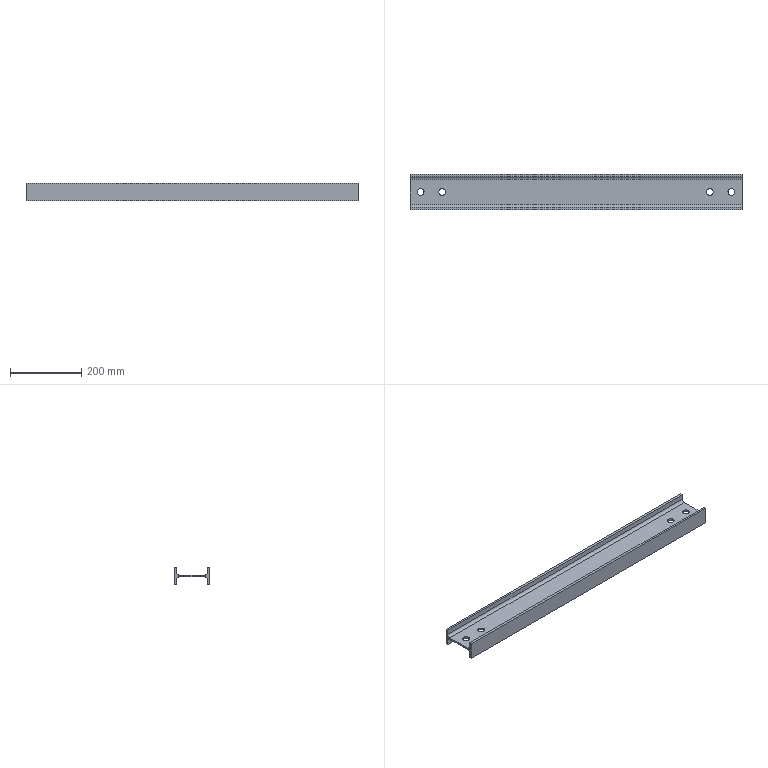Part | STEP file | 计量辅梁10主体_Default<As Machined> | 1 solid | 26 faces | box 932.5 x 100 x 50 mm | volume 1099284 mm3 | plane 14 | cylinder 12 | commonest cylinder face diameters 19 x8 16 x4